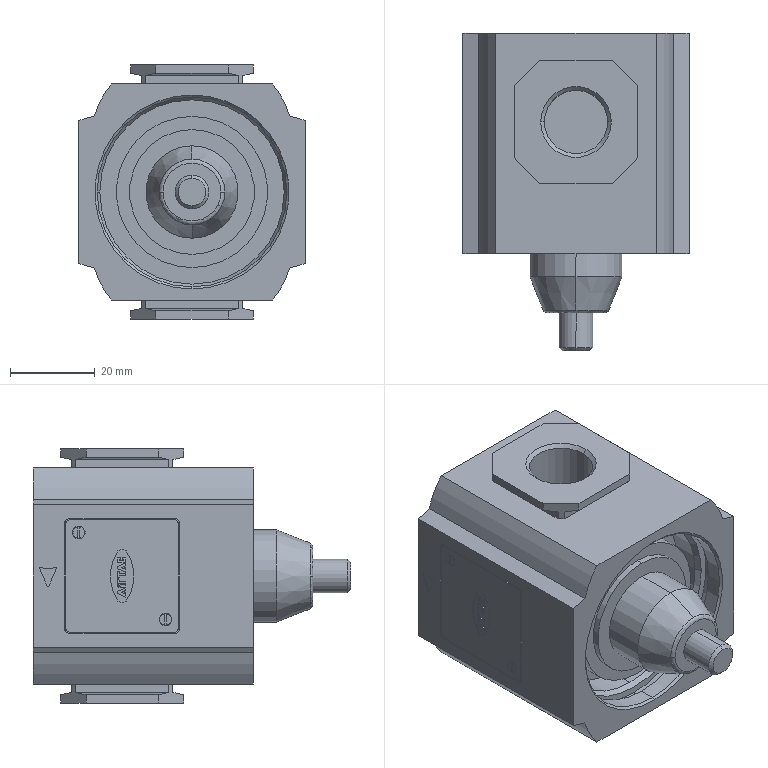Part | SolidWorks | features BaseBody 1 | 1 solid | 255 faces | box 53.4 x 75 x 60 mm | volume 124215 mm3 | plane 144 | cylinder 95 | cone 12 | torus 4 | commonest cylinder face diameters 2 x8 3 x8 4 x8 0.4 x7 0.488 x6 0.543 x5